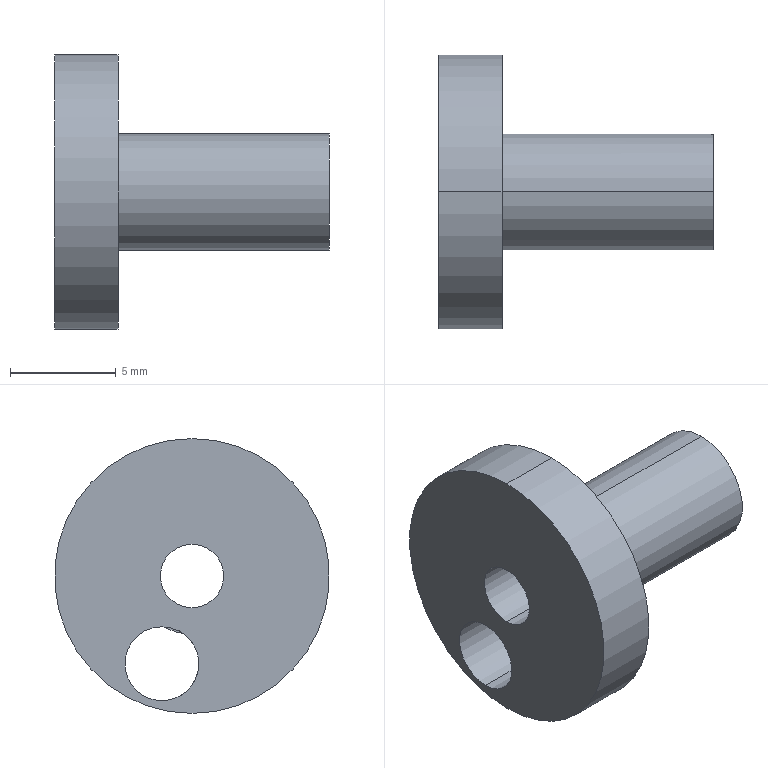Part | STEP file | fiber optic seat 2 | 1 solid | 12 faces | box 13 x 13 x 13 mm | volume 515.025 mm3 | cylinder 8 | plane 4 | commonest cylinder face diameters 3 x2 3.5 x2 5.5 x2 13 x2
STEP:
#1=CARTESIAN_POINT('',(0.,0.,0.));
#2=DIRECTION('',(0.,0.,1.));
#3=DIRECTION('',(1.,0.,0.));
#4=AXIS2_PLACEMENT_3D('',#1,#2,#3);
#5=CARTESIAN_POINT('',(8.087,0.4186,-2.718));
#6=VERTEX_POINT('',#5);
#7=CARTESIAN_POINT('',(8.087,1.339,-2.402));
#8=VERTEX_POINT('',#7);
#9=CARTESIAN_POINT('',(8.087,1.424,-4.15));
#10=DIRECTION('',(-1.,0.,0.));
#11=DIRECTION('',(0.,0.,1.));
#12=AXIS2_PLACEMENT_3D('',#9,#10,#11);
#13=CIRCLE('',#12,1.75);
#14=CARTESIAN_POINT('',(8.087,1.424,-4.15));
#15=DIRECTION('',(-1.,0.,0.));
#16=DIRECTION('',(0.,0.,1.));
#17=AXIS2_PLACEMENT_3D('',#14,#15,#16);
#18=CYLINDRICAL_SURFACE('',#17,1.75);
#19=CARTESIAN_POINT('',(0.,0.));
#20=DIRECTION('',(1.,0.));
#21=VECTOR('',#20,1.);
#22=LINE('',#19,#21);
#23=(GEOMETRIC_REPRESENTATION_CONTEXT(2)PARAMETRIC_REPRESENTATION_CONTEXT()REPRESENTATION_CONTEXT('',''));
#24=DEFINITIONAL_REPRESENTATION('',(#22),#23);
#25=PCURVE('',#18,#24);
#26=CARTESIAN_POINT('',(8.087,1.424,-4.15));
#27=DIRECTION('',(-1.,0.,0.));
#28=DIRECTION('',(0.,0.,1.));
#29=AXIS2_PLACEMENT_3D('',#26,#27,#28);
#30=PLANE('',#29);
#31=CARTESIAN_POINT('',(0.,0.));
#32=DIRECTION('',(1.,0.));
#33=AXIS2_PLACEMENT_2D('',#31,#32);
#34=CIRCLE('',#33,1.75);
#35=(GEOMETRIC_REPRESENTATION_CONTEXT(2)PARAMETRIC_REPRESENTATION_CONTEXT()REPRESENTATION_CONTEXT('',''));
#36=DEFINITIONAL_REPRESENTATION('',(#34),#35);
#37=PCURVE('',#30,#36);
#38=SURFACE_CURVE('',#13,(#25,#37),.PCURVE_S1.);
#39=EDGE_CURVE('',#6,#8,#38,.T.);
#40=ORIENTED_EDGE('',*,*,#39,.T.);
#41=CARTESIAN_POINT('',(8.087,1.424,-2.4));
#42=VERTEX_POINT('',#41);
#43=CARTESIAN_POINT('',(8.087,1.424,-4.15));
#44=DIRECTION('',(-1.,0.,0.));
#45=DIRECTION('',(0.,0.,1.));
#46=AXIS2_PLACEMENT_3D('',#43,#44,#45);
#47=CIRCLE('',#46,1.75);
#48=CARTESIAN_POINT('',(0.,0.));
#49=DIRECTION('',(1.,0.));
#50=VECTOR('',#49,1.);
#51=LINE('',#48,#50);
#52=(GEOMETRIC_REPRESENTATION_CONTEXT(2)PARAMETRIC_REPRESENTATION_CONTEXT()REPRESENTATION_CONTEXT('',''));
#53=DEFINITIONAL_REPRESENTATION('',(#51),#52);
#54=PCURVE('',#18,#53);
#55=CARTESIAN_POINT('',(8.087,2.75,0.));
#56=DIRECTION('',(-1.,0.,0.));
#57=DIRECTION('',(0.,0.,1.));
#58=AXIS2_PLACEMENT_3D('',#55,#56,#57);
#59=PLANE('',#58);
#60=CARTESIAN_POINT('',(-4.15,-1.326));
#61=DIRECTION('',(1.,0.));
#62=AXIS2_PLACEMENT_2D('',#60,#61);
#63=CIRCLE('',#62,1.75);
#64=(GEOMETRIC_REPRESENTATION_CONTEXT(2)PARAMETRIC_REPRESENTATION_CONTEXT()REPRESENTATION_CONTEXT('',''));
#65=DEFINITIONAL_REPRESENTATION('',(#63),#64);
#66=PCURVE('',#59,#65);
#67=SURFACE_CURVE('',#47,(#54,#66),.PCURVE_S1.);
#68=EDGE_CURVE('',#8,#42,#67,.T.);
#69=ORIENTED_EDGE('',*,*,#68,.T.);
#70=CARTESIAN_POINT('',(5.087,1.424,-2.4));
#71=VERTEX_POINT('',#70);
#72=CARTESIAN_POINT('',(8.087,1.424,-2.4));
#73=DIRECTION('',(-1.,0.,0.));
#74=VECTOR('',#73,1.);
#75=LINE('',#72,#74);
#76=CARTESIAN_POINT('',(6.283,0.));
#77=DIRECTION('',(0.,1.));
#78=VECTOR('',#77,1.);
#79=LINE('',#76,#78);
#80=(GEOMETRIC_REPRESENTATION_CONTEXT(2)PARAMETRIC_REPRESENTATION_CONTEXT()REPRESENTATION_CONTEXT('',''));
#81=DEFINITIONAL_REPRESENTATION('',(#79),#80);
#82=PCURVE('',#18,#81);
#83=CARTESIAN_POINT('',(8.087,1.424,-4.15));
#84=DIRECTION('',(-1.,0.,0.));
#85=DIRECTION('',(0.,0.,1.));
#86=AXIS2_PLACEMENT_3D('',#83,#84,#85);
#87=CYLINDRICAL_SURFACE('',#86,1.75);
#88=CARTESIAN_POINT('',(0.,0.));
#89=DIRECTION('',(0.,1.));
#90=VECTOR('',#89,1.);
#91=LINE('',#88,#90);
#92=(GEOMETRIC_REPRESENTATION_CONTEXT(2)PARAMETRIC_REPRESENTATION_CONTEXT()REPRESENTATION_CONTEXT('',''));
#93=DEFINITIONAL_REPRESENTATION('',(#91),#92);
#94=PCURVE('',#87,#93);
#95=SURFACE_CURVE('',#75,(#82,#94),.PCURVE_S1.);
#96=EDGE_CURVE('',#42,#71,#95,.T.);
#97=ORIENTED_EDGE('',*,*,#96,.T.);
#98=CARTESIAN_POINT('',(5.087,1.424,-5.9));
#99=VERTEX_POINT('',#98);
#100=CARTESIAN_POINT('',(5.087,1.424,-4.15));
#101=DIRECTION('',(-1.,0.,0.));
#102=DIRECTION('',(0.,0.,1.));
#103=AXIS2_PLACEMENT_3D('',#100,#101,#102);
#104=CIRCLE('',#103,1.75);
#105=CARTESIAN_POINT('',(0.,3.));
#106=DIRECTION('',(1.,0.));
#107=VECTOR('',#106,1.);
#108=LINE('',#105,#107);
#109=(GEOMETRIC_REPRESENTATION_CONTEXT(2)PARAMETRIC_REPRESENTATION_CONTEXT()REPRESENTATION_CONTEXT('',''));
#110=DEFINITIONAL_REPRESENTATION('',(#108),#109);
#111=PCURVE('',#18,#110);
#112=CARTESIAN_POINT('',(5.087,1.5,0.));
#113=DIRECTION('',(1.,0.,0.));
#114=DIRECTION('',(0.,0.,-1.));
#115=AXIS2_PLACEMENT_3D('',#112,#113,#114);
#116=PLANE('',#115);
#117=CARTESIAN_POINT('',(2.4,-0.07556));
#118=CARTESIAN_POINT('',(2.4,2.956));
#119=CARTESIAN_POINT('',(5.025,1.44));
#120=CARTESIAN_POINT('',(7.65,-0.07556));
#121=CARTESIAN_POINT('',(5.025,-1.591));
#122=CARTESIAN_POINT('',(2.4,-3.107));
#123=CARTESIAN_POINT('',(2.4,-0.07556));
#124=(BOUNDED_CURVE()B_SPLINE_CURVE(2,(#117,#118,#119,#120,#121,#122,#123),.UNSPECIFIED.,.T.,.F.)B_SPLINE_CURVE_WITH_KNOTS((1,2,2,2,2,1),(-2.094,0.,2.094,4.189,6.283,8.378),.UNSPECIFIED.)CURVE()GEOMETRIC_REPRESENTATION_ITEM()RATIONAL_B_SPLINE_CURVE((1.,0.5,1.,0.5,1.,0.5,1.))REPRESENTATION_ITEM(''));
#125=(GEOMETRIC_REPRESENTATION_CONTEXT(2)PARAMETRIC_REPRESENTATION_CONTEXT()REPRESENTATION_CONTEXT('',''));
#126=DEFINITIONAL_REPRESENTATION('',(#124),#125);
#127=PCURVE('',#116,#126);
#128=SURFACE_CURVE('',#104,(#111,#127),.PCURVE_S1.);
#129=EDGE_CURVE('',#99,#71,#128,.T.);
#130=ORIENTED_EDGE('',*,*,#129,.F.);
#131=CARTESIAN_POINT('',(8.087,1.424,-5.9));
#132=VERTEX_POINT('',#131);
#133=CARTESIAN_POINT('',(8.087,1.424,-5.9));
#134=DIRECTION('',(-1.,0.,0.));
#135=VECTOR('',#134,1.);
#136=LINE('',#133,#135);
#137=CARTESIAN_POINT('',(3.142,0.));
#138=DIRECTION('',(0.,1.));
#139=VECTOR('',#138,1.);
#140=LINE('',#137,#139);
#141=(GEOMETRIC_REPRESENTATION_CONTEXT(2)PARAMETRIC_REPRESENTATION_CONTEXT()REPRESENTATION_CONTEXT('',''));
#142=DEFINITIONAL_REPRESENTATION('',(#140),#141);
#143=PCURVE('',#18,#142);
#144=CARTESIAN_POINT('',(3.142,0.));
#145=DIRECTION('',(0.,1.));
#146=VECTOR('',#145,1.);
#147=LINE('',#144,#146);
#148=(GEOMETRIC_REPRESENTATION_CONTEXT(2)PARAMETRIC_REPRESENTATION_CONTEXT()REPRESENTATION_CONTEXT('',''));
#149=DEFINITIONAL_REPRESENTATION('',(#147),#148);
#150=PCURVE('',#87,#149);
#151=SURFACE_CURVE('',#136,(#143,#150),.PCURVE_S1.);
#152=EDGE_CURVE('',#132,#99,#151,.T.);
#153=ORIENTED_EDGE('',*,*,#152,.F.);
#154=CARTESIAN_POINT('',(8.087,1.424,-4.15));
#155=DIRECTION('',(-1.,0.,0.));
#156=DIRECTION('',(0.,0.,1.));
#157=AXIS2_PLACEMENT_3D('',#154,#155,#156);
#158=CIRCLE('',#157,1.75);
#159=CARTESIAN_POINT('',(0.,0.));
#160=DIRECTION('',(1.,0.));
#161=VECTOR('',#160,1.);
#162=LINE('',#159,#161);
#163=(GEOMETRIC_REPRESENTATION_CONTEXT(2)PARAMETRIC_REPRESENTATION_CONTEXT()REPRESENTATION_CONTEXT('',''));
#164=DEFINITIONAL_REPRESENTATION('',(#162),#163);
#165=PCURVE('',#18,#164);
#166=CARTESIAN_POINT('',(-4.15,-1.326));
#167=DIRECTION('',(1.,0.));
#168=AXIS2_PLACEMENT_2D('',#166,#167);
#169=CIRCLE('',#168,1.75);
#170=(GEOMETRIC_REPRESENTATION_CONTEXT(2)PARAMETRIC_REPRESENTATION_CONTEXT()REPRESENTATION_CONTEXT('',''));
#171=DEFINITIONAL_REPRESENTATION('',(#169),#170);
#172=PCURVE('',#59,#171);
#173=SURFACE_CURVE('',#158,(#165,#172),.PCURVE_S1.);
#174=EDGE_CURVE('',#132,#6,#173,.T.);
#175=ORIENTED_EDGE('',*,*,#174,.T.);
#176=EDGE_LOOP('',(#40,#69,#97,#130,#153,#175));
#177=FACE_BOUND('',#176,.F.);
#178=ADVANCED_FACE('',(#177),#18,.F.);
#179=CARTESIAN_POINT('',(18.087,0.,1.5));
#180=VERTEX_POINT('',#179);
#181=CARTESIAN_POINT('',(5.087,0.,1.5));
#182=VERTEX_POINT('',#181);
#183=CARTESIAN_POINT('',(0.,0.,1.5));
#184=DIRECTION('',(-1.,0.,0.));
#185=VECTOR('',#184,1.);
#186=LINE('',#183,#185);
#187=CARTESIAN_POINT('',(0.,0.,0.));
#188=DIRECTION('',(-1.,0.,0.));
#189=DIRECTION('',(0.,0.,1.));
#190=AXIS2_PLACEMENT_3D('',#187,#188,#189);
#191=CYLINDRICAL_SURFACE('',#190,1.5);
#192=CARTESIAN_POINT('',(6.283,0.));
#193=DIRECTION('',(0.,1.));
#194=VECTOR('',#193,1.);
#195=LINE('',#192,#194);
#196=(GEOMETRIC_REPRESENTATION_CONTEXT(2)PARAMETRIC_REPRESENTATION_CONTEXT()REPRESENTATION_CONTEXT('',''));
#197=DEFINITIONAL_REPRESENTATION('',(#195),#196);
#198=PCURVE('',#191,#197);
#199=CARTESIAN_POINT('',(0.,0.,0.));
#200=DIRECTION('',(-1.,0.,0.));
#201=DIRECTION('',(0.,0.,1.));
#202=AXIS2_PLACEMENT_3D('',#199,#200,#201);
#203=CYLINDRICAL_SURFACE('',#202,1.5);
#204=CARTESIAN_POINT('',(0.,0.));
#205=DIRECTION('',(0.,1.));
#206=VECTOR('',#205,1.);
#207=LINE('',#204,#206);
#208=(GEOMETRIC_REPRESENTATION_CONTEXT(2)PARAMETRIC_REPRESENTATION_CONTEXT()REPRESENTATION_CONTEXT('',''));
#209=DEFINITIONAL_REPRESENTATION('',(#207),#208);
#210=PCURVE('',#203,#209);
#211=SURFACE_CURVE('',#186,(#198,#210),.PCURVE_S1.);
#212=EDGE_CURVE('',#180,#182,#211,.T.);
#213=ORIENTED_EDGE('',*,*,#212,.T.);
#214=CARTESIAN_POINT('',(5.087,0.,-1.5));
#215=VERTEX_POINT('',#214);
#216=CARTESIAN_POINT('',(5.087,0.,0.));
#217=DIRECTION('',(-1.,0.,0.));
#218=DIRECTION('',(0.,0.,1.));
#219=AXIS2_PLACEMENT_3D('',#216,#217,#218);
#220=CIRCLE('',#219,1.5);
#221=CARTESIAN_POINT('',(0.,-5.087));
#222=DIRECTION('',(1.,0.));
#223=VECTOR('',#222,1.);
#224=LINE('',#221,#223);
#225=(GEOMETRIC_REPRESENTATION_CONTEXT(2)PARAMETRIC_REPRESENTATION_CONTEXT()REPRESENTATION_CONTEXT('',''));
#226=DEFINITIONAL_REPRESENTATION('',(#224),#225);
#227=PCURVE('',#191,#226);
#228=CARTESIAN_POINT('',(-1.5,-1.5));
#229=CARTESIAN_POINT('',(-1.5,1.098));
#230=CARTESIAN_POINT('',(0.75,-0.201));
#231=CARTESIAN_POINT('',(3.,-1.5));
#232=CARTESIAN_POINT('',(0.75,-2.799));
#233=CARTESIAN_POINT('',(-1.5,-4.098));
#234=CARTESIAN_POINT('',(-1.5,-1.5));
#235=(BOUNDED_CURVE()B_SPLINE_CURVE(2,(#228,#229,#230,#231,#232,#233,#234),.UNSPECIFIED.,.T.,.F.)B_SPLINE_CURVE_WITH_KNOTS((1,2,2,2,2,1),(-2.094,0.,2.094,4.189,6.283,8.378),.UNSPECIFIED.)CURVE()GEOMETRIC_REPRESENTATION_ITEM()RATIONAL_B_SPLINE_CURVE((1.,0.5,1.,0.5,1.,0.5,1.))REPRESENTATION_ITEM(''));
#236=(GEOMETRIC_REPRESENTATION_CONTEXT(2)PARAMETRIC_REPRESENTATION_CONTEXT()REPRESENTATION_CONTEXT('',''));
#237=DEFINITIONAL_REPRESENTATION('',(#235),#236);
#238=PCURVE('',#116,#237);
#239=SURFACE_CURVE('',#220,(#227,#238),.PCURVE_S1.);
#240=EDGE_CURVE('',#215,#182,#239,.T.);
#241=ORIENTED_EDGE('',*,*,#240,.F.);
#242=CARTESIAN_POINT('',(18.087,0.,-1.5));
#243=VERTEX_POINT('',#242);
#244=CARTESIAN_POINT('',(0.,0.,-1.5));
#245=DIRECTION('',(-1.,0.,0.));
#246=VECTOR('',#245,1.);
#247=LINE('',#244,#246);
#248=CARTESIAN_POINT('',(3.142,0.));
#249=DIRECTION('',(0.,1.));
#250=VECTOR('',#249,1.);
#251=LINE('',#248,#250);
#252=(GEOMETRIC_REPRESENTATION_CONTEXT(2)PARAMETRIC_REPRESENTATION_CONTEXT()REPRESENTATION_CONTEXT('',''));
#253=DEFINITIONAL_REPRESENTATION('',(#251),#252);
#254=PCURVE('',#191,#253);
#255=CARTESIAN_POINT('',(3.142,0.));
#256=DIRECTION('',(0.,1.));
#257=VECTOR('',#256,1.);
#258=LINE('',#255,#257);
#259=(GEOMETRIC_REPRESENTATION_CONTEXT(2)PARAMETRIC_REPRESENTATION_CONTEXT()REPRESENTATION_CONTEXT('',''));
#260=DEFINITIONAL_REPRESENTATION('',(#258),#259);
#261=PCURVE('',#203,#260);
#262=SURFACE_CURVE('',#247,(#254,#261),.PCURVE_S1.);
#263=EDGE_CURVE('',#243,#215,#262,.T.);
#264=ORIENTED_EDGE('',*,*,#263,.F.);
#265=CARTESIAN_POINT('',(18.087,0.,0.));
#266=DIRECTION('',(-1.,0.,0.));
#267=DIRECTION('',(0.,0.,1.));
#268=AXIS2_PLACEMENT_3D('',#265,#266,#267);
#269=CIRCLE('',#268,1.5);
#270=CARTESIAN_POINT('',(0.,-18.087));
#271=DIRECTION('',(1.,0.));
#272=VECTOR('',#271,1.);
#273=LINE('',#270,#272);
#274=(GEOMETRIC_REPRESENTATION_CONTEXT(2)PARAMETRIC_REPRESENTATION_CONTEXT()REPRESENTATION_CONTEXT('',''));
#275=DEFINITIONAL_REPRESENTATION('',(#273),#274);
#276=PCURVE('',#191,#275);
#277=CARTESIAN_POINT('',(18.087,1.5,0.));
#278=DIRECTION('',(-1.,0.,0.));
#279=DIRECTION('',(0.,0.,1.));
#280=AXIS2_PLACEMENT_3D('',#277,#278,#279);
#281=PLANE('',#280);
#282=CARTESIAN_POINT('',(0.,-1.5));
#283=DIRECTION('',(1.,0.));
#284=AXIS2_PLACEMENT_2D('',#282,#283);
#285=CIRCLE('',#284,1.5);
#286=(GEOMETRIC_REPRESENTATION_CONTEXT(2)PARAMETRIC_REPRESENTATION_CONTEXT()REPRESENTATION_CONTEXT('',''));
#287=DEFINITIONAL_REPRESENTATION('',(#285),#286);
#288=PCURVE('',#281,#287);
#289=SURFACE_CURVE('',#269,(#276,#288),.PCURVE_S1.);
#290=EDGE_CURVE('',#243,#180,#289,.T.);
#291=ORIENTED_EDGE('',*,*,#290,.T.);
#292=EDGE_LOOP('',(#213,#241,#264,#291));
#293=FACE_BOUND('',#292,.F.);
#294=ADVANCED_FACE('',(#293),#191,.F.);
#295=CARTESIAN_POINT('',(18.087,0.,2.75));
#296=VERTEX_POINT('',#295);
#297=CARTESIAN_POINT('',(18.087,0.,-2.75));
#298=VERTEX_POINT('',#297);
#299=CARTESIAN_POINT('',(18.087,0.,0.));
#300=DIRECTION('',(-1.,0.,0.));
#301=DIRECTION('',(0.,0.,1.));
#302=AXIS2_PLACEMENT_3D('',#299,#300,#301);
#303=CIRCLE('',#302,2.75);
#304=CARTESIAN_POINT('',(0.,0.,0.));
#305=DIRECTION('',(-1.,0.,0.));
#306=DIRECTION('',(0.,0.,1.));
#307=AXIS2_PLACEMENT_3D('',#304,#305,#306);
#308=CYLINDRICAL_SURFACE('',#307,2.75);
#309=CARTESIAN_POINT('',(0.,-18.087));
#310=DIRECTION('',(1.,0.));
#311=VECTOR('',#310,1.);
#312=LINE('',#309,#311);
#313=(GEOMETRIC_REPRESENTATION_CONTEXT(2)PARAMETRIC_REPRESENTATION_CONTEXT()REPRESENTATION_CONTEXT('',''));
#314=DEFINITIONAL_REPRESENTATION('',(#312),#313);
#315=PCURVE('',#308,#314);
#316=CARTESIAN_POINT('',(0.,-1.5));
#317=DIRECTION('',(1.,0.));
#318=AXIS2_PLACEMENT_2D('',#316,#317);
#319=CIRCLE('',#318,2.75);
#320=(GEOMETRIC_REPRESENTATION_CONTEXT(2)PARAMETRIC_REPRESENTATION_CONTEXT()REPRESENTATION_CONTEXT('',''));
#321=DEFINITIONAL_REPRESENTATION('',(#319),#320);
#322=PCURVE('',#281,#321);
#323=SURFACE_CURVE('',#303,(#315,#322),.PCURVE_S1.);
#324=EDGE_CURVE('',#296,#298,#323,.T.);
#325=ORIENTED_EDGE('',*,*,#324,.T.);
#326=CARTESIAN_POINT('',(8.087,0.,-2.75));
#327=VERTEX_POINT('',#326);
#328=CARTESIAN_POINT('',(0.,0.,-2.75));
#329=DIRECTION('',(-1.,0.,0.));
#330=VECTOR('',#329,1.);
#331=LINE('',#328,#330);
#332=CARTESIAN_POINT('',(3.142,0.));
#333=DIRECTION('',(0.,1.));
#334=VECTOR('',#333,1.);
#335=LINE('',#332,#334);
#336=(GEOMETRIC_REPRESENTATION_CONTEXT(2)PARAMETRIC_REPRESENTATION_CONTEXT()REPRESENTATION_CONTEXT('',''));
#337=DEFINITIONAL_REPRESENTATION('',(#335),#336);
#338=PCURVE('',#308,#337);
#339=CARTESIAN_POINT('',(0.,0.,0.));
#340=DIRECTION('',(-1.,0.,0.));
#341=DIRECTION('',(0.,0.,1.));
#342=AXIS2_PLACEMENT_3D('',#339,#340,#341);
#343=CYLINDRICAL_SURFACE('',#342,2.75);
#344=CARTESIAN_POINT('',(3.142,0.));
#345=DIRECTION('',(0.,1.));
#346=VECTOR('',#345,1.);
#347=LINE('',#344,#346);
#348=(GEOMETRIC_REPRESENTATION_CONTEXT(2)PARAMETRIC_REPRESENTATION_CONTEXT()REPRESENTATION_CONTEXT('',''));
#349=DEFINITIONAL_REPRESENTATION('',(#347),#348);
#350=PCURVE('',#343,#349);
#351=SURFACE_CURVE('',#331,(#338,#350),.PCURVE_S1.);
#352=EDGE_CURVE('',#298,#327,#351,.T.);
#353=ORIENTED_EDGE('',*,*,#352,.T.);
#354=CARTESIAN_POINT('',(8.087,0.,0.));
#355=DIRECTION('',(-1.,0.,0.));
#356=DIRECTION('',(0.,0.,1.));
#357=AXIS2_PLACEMENT_3D('',#354,#355,#356);
#358=CIRCLE('',#357,2.75);
#359=CARTESIAN_POINT('',(0.,-8.087));
#360=DIRECTION('',(1.,0.));
#361=VECTOR('',#360,1.);
#362=LINE('',#359,#361);
#363=(GEOMETRIC_REPRESENTATION_CONTEXT(2)PARAMETRIC_REPRESENTATION_CONTEXT()REPRESENTATION_CONTEXT('',''));
#364=DEFINITIONAL_REPRESENTATION('',(#362),#363);
#365=PCURVE('',#308,#364);
#366=CARTESIAN_POINT('',(0.,-2.75));
#367=DIRECTION('',(1.,0.));
#368=AXIS2_PLACEMENT_2D('',#366,#367);
#369=CIRCLE('',#368,2.75);
#370=(GEOMETRIC_REPRESENTATION_CONTEXT(2)PARAMETRIC_REPRESENTATION_CONTEXT()REPRESENTATION_CONTEXT('',''));
#371=DEFINITIONAL_REPRESENTATION('',(#369),#370);
#372=PCURVE('',#59,#371);
#373=SURFACE_CURVE('',#358,(#365,#372),.PCURVE_S1.);
#374=EDGE_CURVE('',#6,#327,#373,.T.);
#375=ORIENTED_EDGE('',*,*,#374,.F.);
#376=CARTESIAN_POINT('',(8.087,0.,0.));
#377=DIRECTION('',(-1.,0.,0.));
#378=DIRECTION('',(0.,0.,1.));
#379=AXIS2_PLACEMENT_3D('',#376,#377,#378);
#380=CIRCLE('',#379,2.75);
#381=CARTESIAN_POINT('',(0.,-8.087));
#382=DIRECTION('',(1.,0.));
#383=VECTOR('',#382,1.);
#384=LINE('',#381,#383);
#385=(GEOMETRIC_REPRESENTATION_CONTEXT(2)PARAMETRIC_REPRESENTATION_CONTEXT()REPRESENTATION_CONTEXT('',''));
#386=DEFINITIONAL_REPRESENTATION('',(#384),#385);
#387=PCURVE('',#308,#386);
#388=CARTESIAN_POINT('',(4.15,-1.424));
#389=DIRECTION('',(1.,0.));
#390=AXIS2_PLACEMENT_2D('',#388,#389);
#391=CIRCLE('',#390,2.75);
#392=(GEOMETRIC_REPRESENTATION_CONTEXT(2)PARAMETRIC_REPRESENTATION_CONTEXT()REPRESENTATION_CONTEXT('',''));
#393=DEFINITIONAL_REPRESENTATION('',(#391),#392);
#394=PCURVE('',#30,#393);
#395=SURFACE_CURVE('',#380,(#387,#394),.PCURVE_S1.);
#396=EDGE_CURVE('',#8,#6,#395,.T.);
#397=ORIENTED_EDGE('',*,*,#396,.F.);
#398=CARTESIAN_POINT('',(8.087,0.,2.75));
#399=VERTEX_POINT('',#398);
#400=CARTESIAN_POINT('',(8.087,0.,0.));
#401=DIRECTION('',(-1.,0.,0.));
#402=DIRECTION('',(0.,0.,1.));
#403=AXIS2_PLACEMENT_3D('',#400,#401,#402);
#404=CIRCLE('',#403,2.75);
#405=CARTESIAN_POINT('',(0.,-8.087));
#406=DIRECTION('',(1.,0.));
#407=VECTOR('',#406,1.);
#408=LINE('',#405,#407);
#409=(GEOMETRIC_REPRESENTATION_CONTEXT(2)PARAMETRIC_REPRESENTATION_CONTEXT()REPRESENTATION_CONTEXT('',''));
#410=DEFINITIONAL_REPRESENTATION('',(#408),#409);
#411=PCURVE('',#308,#410);
#412=CARTESIAN_POINT('',(0.,-2.75));
#413=DIRECTION('',(1.,0.));
#414=AXIS2_PLACEMENT_2D('',#412,#413);
#415=CIRCLE('',#414,2.75);
#416=(GEOMETRIC_REPRESENTATION_CONTEXT(2)PARAMETRIC_REPRESENTATION_CONTEXT()REPRESENTATION_CONTEXT('',''));
#417=DEFINITIONAL_REPRESENTATION('',(#415),#416);
#418=PCURVE('',#59,#417);
#419=SURFACE_CURVE('',#404,(#411,#418),.PCURVE_S1.);
#420=EDGE_CURVE('',#399,#8,#419,.T.);
#421=ORIENTED_EDGE('',*,*,#420,.F.);
#422=CARTESIAN_POINT('',(0.,0.,2.75));
#423=DIRECTION('',(-1.,0.,0.));
#424=VECTOR('',#423,1.);
#425=LINE('',#422,#424);
#426=CARTESIAN_POINT('',(0.,0.));
#427=DIRECTION('',(0.,1.));
#428=VECTOR('',#427,1.);
#429=LINE('',#426,#428);
#430=(GEOMETRIC_REPRESENTATION_CONTEXT(2)PARAMETRIC_REPRESENTATION_CONTEXT()REPRESENTATION_CONTEXT('',''));
#431=DEFINITIONAL_REPRESENTATION('',(#429),#430);
#432=PCURVE('',#308,#431);
#433=CARTESIAN_POINT('',(6.283,0.));
#434=DIRECTION('',(0.,1.));
#435=VECTOR('',#434,1.);
#436=LINE('',#433,#435);
#437=(GEOMETRIC_REPRESENTATION_CONTEXT(2)PARAMETRIC_REPRESENTATION_CONTEXT()REPRESENTATION_CONTEXT('',''));
#438=DEFINITIONAL_REPRESENTATION('',(#436),#437);
#439=PCURVE('',#343,#438);
#440=SURFACE_CURVE('',#425,(#432,#439),.PCURVE_S1.);
#441=EDGE_CURVE('',#296,#399,#440,.T.);
#442=ORIENTED_EDGE('',*,*,#441,.F.);
#443=EDGE_LOOP('',(#325,#353,#375,#397,#421,#442));
#444=FACE_BOUND('',#443,.T.);
#445=ADVANCED_FACE('',(#444),#308,.T.);
#446=CARTESIAN_POINT('',(8.087,0.,6.5));
#447=VERTEX_POINT('',#446);
#448=CARTESIAN_POINT('',(8.087,0.,-6.5));
#449=VERTEX_POINT('',#448);
#450=CARTESIAN_POINT('',(8.087,0.,0.));
#451=DIRECTION('',(-1.,0.,0.));
#452=DIRECTION('',(0.,0.,1.));
#453=AXIS2_PLACEMENT_3D('',#450,#451,#452);
#454=CIRCLE('',#453,6.5);
#455=CARTESIAN_POINT('',(0.,0.,0.));
#456=DIRECTION('',(-1.,0.,0.));
#457=DIRECTION('',(0.,0.,1.));
#458=AXIS2_PLACEMENT_3D('',#455,#456,#457);
#459=CYLINDRICAL_SURFACE('',#458,6.5);
#460=CARTESIAN_POINT('',(0.,-8.087));
#461=DIRECTION('',(1.,0.));
#462=VECTOR('',#461,1.);
#463=LINE('',#460,#462);
#464=(GEOMETRIC_REPRESENTATION_CONTEXT(2)PARAMETRIC_REPRESENTATION_CONTEXT()REPRESENTATION_CONTEXT('',''));
#465=DEFINITIONAL_REPRESENTATION('',(#463),#464);
#466=PCURVE('',#459,#465);
#467=CARTESIAN_POINT('',(0.,-2.75));
#468=DIRECTION('',(1.,0.));
#469=AXIS2_PLACEMENT_2D('',#467,#468);
#470=CIRCLE('',#469,6.5);
#471=(GEOMETRIC_REPRESENTATION_CONTEXT(2)PARAMETRIC_REPRESENTATION_CONTEXT()REPRESENTATION_CONTEXT('',''));
#472=DEFINITIONAL_REPRESENTATION('',(#470),#471);
#473=PCURVE('',#59,#472);
#474=SURFACE_CURVE('',#454,(#466,#473),.PCURVE_S1.);
#475=EDGE_CURVE('',#447,#449,#474,.T.);
#476=ORIENTED_EDGE('',*,*,#475,.T.);
#477=CARTESIAN_POINT('',(5.087,0.,-6.5));
#478=VERTEX_POINT('',#477);
#479=CARTESIAN_POINT('',(0.,0.,-6.5));
#480=DIRECTION('',(-1.,0.,0.));
#481=VECTOR('',#480,1.);
#482=LINE('',#479,#481);
#483=CARTESIAN_POINT('',(3.142,0.));
#484=DIRECTION('',(0.,1.));
#485=VECTOR('',#484,1.);
#486=LINE('',#483,#485);
#487=(GEOMETRIC_REPRESENTATION_CONTEXT(2)PARAMETRIC_REPRESENTATION_CONTEXT()REPRESENTATION_CONTEXT('',''));
#488=DEFINITIONAL_REPRESENTATION('',(#486),#487);
#489=PCURVE('',#459,#488);
#490=CARTESIAN_POINT('',(0.,0.,0.));
#491=DIRECTION('',(-1.,0.,0.));
#492=DIRECTION('',(0.,0.,1.));
#493=AXIS2_PLACEMENT_3D('',#490,#491,#492);
#494=CYLINDRICAL_SURFACE('',#493,6.5);
#495=CARTESIAN_POINT('',(3.142,0.));
#496=DIRECTION('',(0.,1.));
#497=VECTOR('',#496,1.);
#498=LINE('',#495,#497);
#499=(GEOMETRIC_REPRESENTATION_CONTEXT(2)PARAMETRIC_REPRESENTATION_CONTEXT()REPRESENTATION_CONTEXT('',''));
#500=DEFINITIONAL_REPRESENTATION('',(#498),#499);
#501=PCURVE('',#494,#500);
#502=SURFACE_CURVE('',#482,(#489,#501),.PCURVE_S1.);
#503=EDGE_CURVE('',#449,#478,#502,.T.);
#504=ORIENTED_EDGE('',*,*,#503,.T.);
#505=CARTESIAN_POINT('',(5.087,0.,6.5));
#506=VERTEX_POINT('',#505);
#507=CARTESIAN_POINT('',(5.087,0.,0.));
#508=DIRECTION('',(-1.,0.,0.));
#509=DIRECTION('',(0.,0.,1.));
#510=AXIS2_PLACEMENT_3D('',#507,#508,#509);
#511=CIRCLE('',#510,6.5);
#512=CARTESIAN_POINT('',(0.,-5.087));
#513=DIRECTION('',(1.,0.));
#514=VECTOR('',#513,1.);
#515=LINE('',#512,#514);
#516=(GEOMETRIC_REPRESENTATION_CONTEXT(2)PARAMETRIC_REPRESENTATION_CONTEXT()REPRESENTATION_CONTEXT('',''));
#517=DEFINITIONAL_REPRESENTATION('',(#515),#516);
#518=PCURVE('',#459,#517);
#519=CARTESIAN_POINT('',(-6.5,-1.5));
#520=CARTESIAN_POINT('',(-6.5,9.758));
#521=CARTESIAN_POINT('',(3.25,4.129));
#522=CARTESIAN_POINT('',(13.,-1.5));
#523=CARTESIAN_POINT('',(3.25,-7.129));
#524=CARTESIAN_POINT('',(-6.5,-12.758));
#525=CARTESIAN_POINT('',(-6.5,-1.5));
#526=(BOUNDED_CURVE()B_SPLINE_CURVE(2,(#519,#520,#521,#522,#523,#524,#525),.UNSPECIFIED.,.T.,.F.)B_SPLINE_CURVE_WITH_KNOTS((1,2,2,2,2,1),(-2.094,0.,2.094,4.189,6.283,8.378),.UNSPECIFIED.)CURVE()GEOMETRIC_REPRESENTATION_ITEM()RATIONAL_B_SPLINE_CURVE((1.,0.5,1.,0.5,1.,0.5,1.))REPRESENTATION_ITEM(''));
#527=(GEOMETRIC_REPRESENTATION_CONTEXT(2)PARAMETRIC_REPRESENTATION_CONTEXT()REPRESENTATION_CONTEXT('',''));
#528=DEFINITIONAL_REPRESENTATION('',(#526),#527);
#529=PCURVE('',#116,#528);
#530=SURFACE_CURVE('',#511,(#518,#529),.PCURVE_S1.);
#531=EDGE_CURVE('',#506,#478,#530,.T.);
#532=ORIENTED_EDGE('',*,*,#531,.F.);
#533=CARTESIAN_POINT('',(0.,0.,6.5));
#534=DIRECTION('',(-1.,0.,0.));
#535=VECTOR('',#534,1.);
#536=LINE('',#533,#535);
#537=CARTESIAN_POINT('',(0.,0.));
#538=DIRECTION('',(0.,1.));
#539=VECTOR('',#538,1.);
#540=LINE('',#537,#539);
#541=(GEOMETRIC_REPRESENTATION_CONTEXT(2)PARAMETRIC_REPRESENTATION_CONTEXT()REPRESENTATION_CONTEXT('',''));
#542=DEFINITIONAL_REPRESENTATION('',(#540),#541);
#543=PCURVE('',#459,#542);
#544=CARTESIAN_POINT('',(6.283,0.));
#545=DIRECTION('',(0.,1.));
#546=VECTOR('',#545,1.);
#547=LINE('',#544,#546);
#548=(GEOMETRIC_REPRESENTATION_CONTEXT(2)PARAMETRIC_REPRESENTATION_CONTEXT()REPRESENTATION_CONTEXT('',''));
#549=DEFINITIONAL_REPRESENTATION('',(#547),#548);
#550=PCURVE('',#494,#549);
#551=SURFACE_CURVE('',#536,(#543,#550),.PCURVE_S1.);
#552=EDGE_CURVE('',#447,#506,#551,.T.);
#553=ORIENTED_EDGE('',*,*,#552,.F.);
#554=EDGE_LOOP('',(#476,#504,#532,#553));
#555=FACE_BOUND('',#554,.T.);
#556=ADVANCED_FACE('',(#555),#459,.T.);
#557=CARTESIAN_POINT('',(5.087,1.424,-4.15));
#558=DIRECTION('',(-1.,0.,0.));
#559=DIRECTION('',(0.,0.,1.));
#560=AXIS2_PLACEMENT_3D('',#557,#558,#559);
#561=CIRCLE('',#560,1.75);
#562=CARTESIAN_POINT('',(2.4,-0.07556));
#563=CARTESIAN_POINT('',(2.4,2.956));
#564=CARTESIAN_POINT('',(5.025,1.44));
#565=CARTESIAN_POINT('',(7.65,-0.07556));
#566=CARTESIAN_POINT('',(5.025,-1.591));
#567=CARTESIAN_POINT('',(2.4,-3.107));
#568=CARTESIAN_POINT('',(2.4,-0.07556));
#569=(BOUNDED_CURVE()B_SPLINE_CURVE(2,(#562,#563,#564,#565,#566,#567,#568),.UNSPECIFIED.,.T.,.F.)B_SPLINE_CURVE_WITH_KNOTS((1,2,2,2,2,1),(-2.094,0.,2.094,4.189,6.283,8.378),.UNSPECIFIED.)CURVE()GEOMETRIC_REPRESENTATION_ITEM()RATIONAL_B_SPLINE_CURVE((1.,0.5,1.,0.5,1.,0.5,1.))REPRESENTATION_ITEM(''));
#570=(GEOMETRIC_REPRESENTATION_CONTEXT(2)PARAMETRIC_REPRESENTATION_CONTEXT()REPRESENTATION_CONTEXT('',''));
#571=DEFINITIONAL_REPRESENTATION('',(#569),#570);
#572=PCURVE('',#116,#571);
#573=CARTESIAN_POINT('',(0.,3.));
#574=DIRECTION('',(1.,0.));
#575=VECTOR('',#574,1.);
#576=LINE('',#573,#575);
#577=(GEOMETRIC_REPRESENTATION_CONTEXT(2)PARAMETRIC_REPRESENTATION_CONTEXT()REPRESENTATION_CONTEXT('',''));
#578=DEFINITIONAL_REPRESENTATION('',(#576),#577);
#579=PCURVE('',#87,#578);
#580=SURFACE_CURVE('',#561,(#572,#579),.PCURVE_S1.);
#581=EDGE_CURVE('',#71,#99,#580,.T.);
#582=ORIENTED_EDGE('',*,*,#581,.F.);
#583=ORIENTED_EDGE('',*,*,#129,.F.);
#584=EDGE_LOOP('',(#582,#583));
#585=FACE_BOUND('',#584,.T.);
#586=CARTESIAN_POINT('',(5.087,0.,0.));
#587=DIRECTION('',(-1.,0.,0.));
#588=DIRECTION('',(0.,0.,1.));
#589=AXIS2_PLACEMENT_3D('',#586,#587,#588);
#590=CIRCLE('',#589,1.5);
#591=CARTESIAN_POINT('',(-1.5,-1.5));
#592=CARTESIAN_POINT('',(-1.5,1.098));
#593=CARTESIAN_POINT('',(0.75,-0.201));
#594=CARTESIAN_POINT('',(3.,-1.5));
#595=CARTESIAN_POINT('',(0.75,-2.799));
#596=CARTESIAN_POINT('',(-1.5,-4.098));
#597=CARTESIAN_POINT('',(-1.5,-1.5));
#598=(BOUNDED_CURVE()B_SPLINE_CURVE(2,(#591,#592,#593,#594,#595,#596,#597),.UNSPECIFIED.,.T.,.F.)B_SPLINE_CURVE_WITH_KNOTS((1,2,2,2,2,1),(-2.094,0.,2.094,4.189,6.283,8.378),.UNSPECIFIED.)CURVE()GEOMETRIC_REPRESENTATION_ITEM()RATIONAL_B_SPLINE_CURVE((1.,0.5,1.,0.5,1.,0.5,1.))REPRESENTATION_ITEM(''));
#599=(GEOMETRIC_REPRESENTATION_CONTEXT(2)PARAMETRIC_REPRESENTATION_CONTEXT()REPRESENTATION_CONTEXT('',''));
#600=DEFINITIONAL_REPRESENTATION('',(#598),#599);
#601=PCURVE('',#116,#600);
#602=CARTESIAN_POINT('',(0.,-5.087));
#603=DIRECTION('',(1.,0.));
#604=VECTOR('',#603,1.);
#605=LINE('',#602,#604);
#606=(GEOMETRIC_REPRESENTATION_CONTEXT(2)PARAMETRIC_REPRESENTATION_CONTEXT()REPRESENTATION_CONTEXT('',''));
#607=DEFINITIONAL_REPRESENTATION('',(#605),#606);
#608=PCURVE('',#203,#607);
#609=SURFACE_CURVE('',#590,(#601,#608),.PCURVE_S1.);
#610=EDGE_CURVE('',#182,#215,#609,.T.);
#611=ORIENTED_EDGE('',*,*,#610,.F.);
#612=ORIENTED_EDGE('',*,*,#240,.F.);
#613=EDGE_LOOP('',(#611,#612));
#614=FACE_BOUND('',#613,.T.);
#615=ORIENTED_EDGE('',*,*,#531,.T.);
#616=CARTESIAN_POINT('',(5.087,0.,0.));
#617=DIRECTION('',(-1.,0.,0.));
#618=DIRECTION('',(0.,0.,1.));
#619=AXIS2_PLACEMENT_3D('',#616,#617,#618);
#620=CIRCLE('',#619,6.5);
#621=CARTESIAN_POINT('',(-6.5,-1.5));
#622=CARTESIAN_POINT('',(-6.5,9.758));
#623=CARTESIAN_POINT('',(3.25,4.129));
#624=CARTESIAN_POINT('',(13.,-1.5));
#625=CARTESIAN_POINT('',(3.25,-7.129));
#626=CARTESIAN_POINT('',(-6.5,-12.758));
#627=CARTESIAN_POINT('',(-6.5,-1.5));
#628=(BOUNDED_CURVE()B_SPLINE_CURVE(2,(#621,#622,#623,#624,#625,#626,#627),.UNSPECIFIED.,.T.,.F.)B_SPLINE_CURVE_WITH_KNOTS((1,2,2,2,2,1),(-2.094,0.,2.094,4.189,6.283,8.378),.UNSPECIFIED.)CURVE()GEOMETRIC_REPRESENTATION_ITEM()RATIONAL_B_SPLINE_CURVE((1.,0.5,1.,0.5,1.,0.5,1.))REPRESENTATION_ITEM(''));
#629=(GEOMETRIC_REPRESENTATION_CONTEXT(2)PARAMETRIC_REPRESENTATION_CONTEXT()REPRESENTATION_CONTEXT('',''));
#630=DEFINITIONAL_REPRESENTATION('',(#628),#629);
#631=PCURVE('',#116,#630);
#632=CARTESIAN_POINT('',(0.,-5.087));
#633=DIRECTION('',(1.,0.));
#634=VECTOR('',#633,1.);
#635=LINE('',#632,#634);
#636=(GEOMETRIC_REPRESENTATION_CONTEXT(2)PARAMETRIC_REPRESENTATION_CONTEXT()REPRESENTATION_CONTEXT('',''));
#637=DEFINITIONAL_REPRESENTATION('',(#635),#636);
#638=PCURVE('',#494,#637);
#639=SURFACE_CURVE('',#620,(#631,#638),.PCURVE_S1.);
#640=EDGE_CURVE('',#478,#506,#639,.T.);
#641=ORIENTED_EDGE('',*,*,#640,.T.);
#642=EDGE_LOOP('',(#615,#641));
#643=FACE_BOUND('',#642,.T.);
#644=ADVANCED_FACE('',(#585,#614,#643),#116,.F.);
#645=ORIENTED_EDGE('',*,*,#503,.F.);
#646=CARTESIAN_POINT('',(8.087,0.,0.));
#647=DIRECTION('',(-1.,0.,0.));
#648=DIRECTION('',(0.,0.,1.));
#649=AXIS2_PLACEMENT_3D('',#646,#647,#648);
#650=CIRCLE('',#649,6.5);
#651=CARTESIAN_POINT('',(0.,-8.087));
#652=DIRECTION('',(1.,0.));
#653=VECTOR('',#652,1.);
#654=LINE('',#651,#653);
#655=(GEOMETRIC_REPRESENTATION_CONTEXT(2)PARAMETRIC_REPRESENTATION_CONTEXT()REPRESENTATION_CONTEXT('',''));
#656=DEFINITIONAL_REPRESENTATION('',(#654),#655);
#657=PCURVE('',#494,#656);
#658=CARTESIAN_POINT('',(0.,-2.75));
#659=DIRECTION('',(1.,0.));
#660=AXIS2_PLACEMENT_2D('',#658,#659);
#661=CIRCLE('',#660,6.5);
#662=(GEOMETRIC_REPRESENTATION_CONTEXT(2)PARAMETRIC_REPRESENTATION_CONTEXT()REPRESENTATION_CONTEXT('',''));
#663=DEFINITIONAL_REPRESENTATION('',(#661),#662);
#664=PCURVE('',#59,#663);
#665=SURFACE_CURVE('',#650,(#657,#664),.PCURVE_S1.);
#666=EDGE_CURVE('',#449,#447,#665,.T.);
#667=ORIENTED_EDGE('',*,*,#666,.T.);
#668=ORIENTED_EDGE('',*,*,#552,.T.);
#669=ORIENTED_EDGE('',*,*,#640,.F.);
#670=EDGE_LOOP('',(#645,#667,#668,#669));
#671=FACE_BOUND('',#670,.T.);
#672=ADVANCED_FACE('',(#671),#494,.T.);
#673=ORIENTED_EDGE('',*,*,#475,.F.);
#674=ORIENTED_EDGE('',*,*,#666,.F.);
#675=EDGE_LOOP('',(#673,#674));
#676=FACE_BOUND('',#675,.T.);
#677=ORIENTED_EDGE('',*,*,#374,.T.);
#678=CARTESIAN_POINT('',(8.087,0.,0.));
#679=DIRECTION('',(-1.,0.,0.));
#680=DIRECTION('',(0.,0.,1.));
#681=AXIS2_PLACEMENT_3D('',#678,#679,#680);
#682=CIRCLE('',#681,2.75);
#683=CARTESIAN_POINT('',(0.,-2.75));
#684=DIRECTION('',(1.,0.));
#685=AXIS2_PLACEMENT_2D('',#683,#684);
#686=CIRCLE('',#685,2.75);
#687=(GEOMETRIC_REPRESENTATION_CONTEXT(2)PARAMETRIC_REPRESENTATION_CONTEXT()REPRESENTATION_CONTEXT('',''));
#688=DEFINITIONAL_REPRESENTATION('',(#686),#687);
#689=PCURVE('',#59,#688);
#690=CARTESIAN_POINT('',(0.,-8.087));
#691=DIRECTION('',(1.,0.));
#692=VECTOR('',#691,1.);
#693=LINE('',#690,#692);
#694=(GEOMETRIC_REPRESENTATION_CONTEXT(2)PARAMETRIC_REPRESENTATION_CONTEXT()REPRESENTATION_CONTEXT('',''));
#695=DEFINITIONAL_REPRESENTATION('',(#693),#694);
#696=PCURVE('',#343,#695);
#697=SURFACE_CURVE('',#682,(#689,#696),.PCURVE_S1.);
#698=EDGE_CURVE('',#327,#399,#697,.T.);
#699=ORIENTED_EDGE('',*,*,#698,.T.);
#700=ORIENTED_EDGE('',*,*,#420,.T.);
#701=ORIENTED_EDGE('',*,*,#68,.T.);
#702=CARTESIAN_POINT('',(8.087,1.424,-4.15));
#703=DIRECTION('',(-1.,0.,0.));
#704=DIRECTION('',(0.,0.,1.));
#705=AXIS2_PLACEMENT_3D('',#702,#703,#704);
#706=CIRCLE('',#705,1.75);
#707=CARTESIAN_POINT('',(-4.15,-1.326));
#708=DIRECTION('',(1.,0.));
#709=AXIS2_PLACEMENT_2D('',#707,#708);
#710=CIRCLE('',#709,1.75);
#711=(GEOMETRIC_REPRESENTATION_CONTEXT(2)PARAMETRIC_REPRESENTATION_CONTEXT()REPRESENTATION_CONTEXT('',''));
#712=DEFINITIONAL_REPRESENTATION('',(#710),#711);
#713=PCURVE('',#59,#712);
#714=CARTESIAN_POINT('',(0.,0.));
#715=DIRECTION('',(1.,0.));
#716=VECTOR('',#715,1.);
#717=LINE('',#714,#716);
#718=(GEOMETRIC_REPRESENTATION_CONTEXT(2)PARAMETRIC_REPRESENTATION_CONTEXT()REPRESENTATION_CONTEXT('',''));
#719=DEFINITIONAL_REPRESENTATION('',(#717),#718);
#720=PCURVE('',#87,#719);
#721=SURFACE_CURVE('',#706,(#713,#720),.PCURVE_S1.);
#722=EDGE_CURVE('',#42,#132,#721,.T.);
#723=ORIENTED_EDGE('',*,*,#722,.T.);
#724=ORIENTED_EDGE('',*,*,#174,.T.);
#725=EDGE_LOOP('',(#677,#699,#700,#701,#723,#724));
#726=FACE_BOUND('',#725,.T.);
#727=ADVANCED_FACE('',(#676,#726),#59,.F.);
#728=ORIENTED_EDGE('',*,*,#352,.F.);
#729=CARTESIAN_POINT('',(18.087,0.,0.));
#730=DIRECTION('',(-1.,0.,0.));
#731=DIRECTION('',(0.,0.,1.));
#732=AXIS2_PLACEMENT_3D('',#729,#730,#731);
#733=CIRCLE('',#732,2.75);
#734=CARTESIAN_POINT('',(0.,-18.087));
#735=DIRECTION('',(1.,0.));
#736=VECTOR('',#735,1.);
#737=LINE('',#734,#736);
#738=(GEOMETRIC_REPRESENTATION_CONTEXT(2)PARAMETRIC_REPRESENTATION_CONTEXT()REPRESENTATION_CONTEXT('',''));
#739=DEFINITIONAL_REPRESENTATION('',(#737),#738);
#740=PCURVE('',#343,#739);
#741=CARTESIAN_POINT('',(0.,-1.5));
#742=DIRECTION('',(1.,0.));
#743=AXIS2_PLACEMENT_2D('',#741,#742);
#744=CIRCLE('',#743,2.75);
#745=(GEOMETRIC_REPRESENTATION_CONTEXT(2)PARAMETRIC_REPRESENTATION_CONTEXT()REPRESENTATION_CONTEXT('',''));
#746=DEFINITIONAL_REPRESENTATION('',(#744),#745);
#747=PCURVE('',#281,#746);
#748=SURFACE_CURVE('',#733,(#740,#747),.PCURVE_S1.);
#749=EDGE_CURVE('',#298,#296,#748,.T.);
#750=ORIENTED_EDGE('',*,*,#749,.T.);
#751=ORIENTED_EDGE('',*,*,#441,.T.);
#752=ORIENTED_EDGE('',*,*,#698,.F.);
#753=EDGE_LOOP('',(#728,#750,#751,#752));
#754=FACE_BOUND('',#753,.T.);
#755=ADVANCED_FACE('',(#754),#343,.T.);
#756=ORIENTED_EDGE('',*,*,#324,.F.);
#757=ORIENTED_EDGE('',*,*,#749,.F.);
#758=EDGE_LOOP('',(#756,#757));
#759=FACE_BOUND('',#758,.T.);
#760=CARTESIAN_POINT('',(18.087,0.,0.));
#761=DIRECTION('',(-1.,0.,0.));
#762=DIRECTION('',(0.,0.,1.));
#763=AXIS2_PLACEMENT_3D('',#760,#761,#762);
#764=CIRCLE('',#763,1.5);
#765=CARTESIAN_POINT('',(0.,-1.5));
#766=DIRECTION('',(1.,0.));
#767=AXIS2_PLACEMENT_2D('',#765,#766);
#768=CIRCLE('',#767,1.5);
#769=(GEOMETRIC_REPRESENTATION_CONTEXT(2)PARAMETRIC_REPRESENTATION_CONTEXT()REPRESENTATION_CONTEXT('',''));
#770=DEFINITIONAL_REPRESENTATION('',(#768),#769);
#771=PCURVE('',#281,#770);
#772=CARTESIAN_POINT('',(0.,-18.087));
#773=DIRECTION('',(1.,0.));
#774=VECTOR('',#773,1.);
#775=LINE('',#772,#774);
#776=(GEOMETRIC_REPRESENTATION_CONTEXT(2)PARAMETRIC_REPRESENTATION_CONTEXT()REPRESENTATION_CONTEXT('',''));
#777=DEFINITIONAL_REPRESENTATION('',(#775),#776);
#778=PCURVE('',#203,#777);
#779=SURFACE_CURVE('',#764,(#771,#778),.PCURVE_S1.);
#780=EDGE_CURVE('',#180,#243,#779,.T.);
#781=ORIENTED_EDGE('',*,*,#780,.T.);
#782=ORIENTED_EDGE('',*,*,#290,.T.);
#783=EDGE_LOOP('',(#781,#782));
#784=FACE_BOUND('',#783,.T.);
#785=ADVANCED_FACE('',(#759,#784),#281,.F.);
#786=ORIENTED_EDGE('',*,*,#610,.F.);
#787=ORIENTED_EDGE('',*,*,#212,.F.);
#788=ORIENTED_EDGE('',*,*,#780,.T.);
#789=ORIENTED_EDGE('',*,*,#263,.T.);
#790=EDGE_LOOP('',(#786,#787,#788,#789));
#791=FACE_BOUND('',#790,.F.);
#792=ADVANCED_FACE('',(#791),#203,.F.);
#793=ORIENTED_EDGE('',*,*,#396,.T.);
#794=ORIENTED_EDGE('',*,*,#39,.T.);
#795=EDGE_LOOP('',(#793,#794));
#796=FACE_BOUND('',#795,.T.);
#797=ADVANCED_FACE('',(#796),#30,.T.);
#798=ORIENTED_EDGE('',*,*,#581,.F.);
#799=ORIENTED_EDGE('',*,*,#96,.F.);
#800=ORIENTED_EDGE('',*,*,#722,.T.);
#801=ORIENTED_EDGE('',*,*,#152,.T.);
#802=EDGE_LOOP('',(#798,#799,#800,#801));
#803=FACE_BOUND('',#802,.F.);
#804=ADVANCED_FACE('',(#803),#87,.F.);
#805=CLOSED_SHELL('',(#178,#294,#445,#556,#644,#672,#727,#755,#785,#792,#797,#804));
#806=MANIFOLD_SOLID_BREP('',#805);
#807=(LENGTH_UNIT()NAMED_UNIT(*)SI_UNIT(.MILLI.,.METRE.));
#808=UNCERTAINTY_MEASURE_WITH_UNIT(LENGTH_MEASURE(0.0000001),#807,'','');
#809=(NAMED_UNIT(*)PLANE_ANGLE_UNIT()SI_UNIT($,.RADIAN.));
#810=(NAMED_UNIT(*)SI_UNIT($,.STERADIAN.)SOLID_ANGLE_UNIT());
#811=(GEOMETRIC_REPRESENTATION_CONTEXT(3)GLOBAL_UNCERTAINTY_ASSIGNED_CONTEXT((#808))GLOBAL_UNIT_ASSIGNED_CONTEXT((#807,#809,#810))REPRESENTATION_CONTEXT('',''));
#812=ADVANCED_BREP_SHAPE_REPRESENTATION('',(#4,#806),#811);